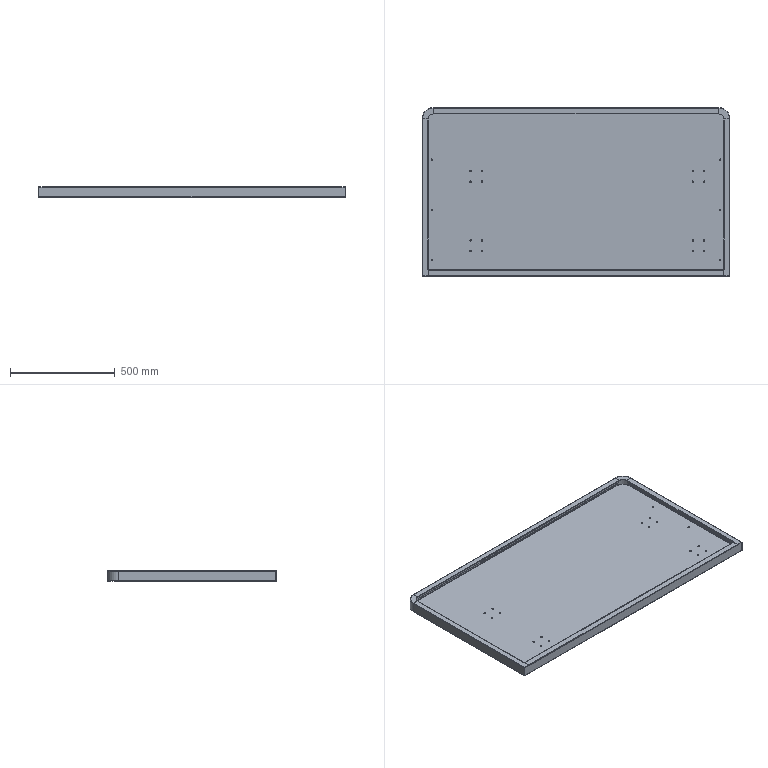Part | SolidWorks | features EdgeFlange 11, 3DProfileFeature 4, Cut 3, LPattern 3, MirrorPattern 2, Fillet 1, FlatPattern 1, SMBaseFlange 1, SheetMetal 1 | 1 solid | 212 faces | box 1469 x 804.6 x 50 mm | volume 2339637 mm3 | plane 126 | cylinder 74 | torus 8 | spline 4 | commonest cylinder face diameters 7 x32 6 x12 1.6 x10 4.6 x10 1.473 x2 4.473 x2